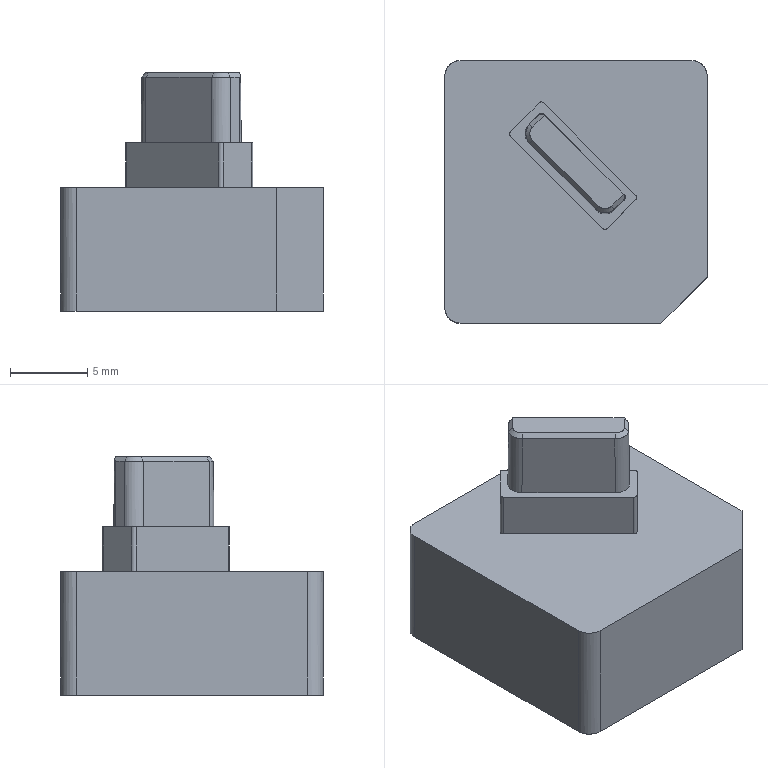NC program | PowerMill | posted with a generic post | part box 17 x 17 x 15.424 mm
Lines 24578 to 24748 of 24748:
N24675 M6
N24676 S15000 M03
N24677 G00 G90 X0.0 Y0.0
N24678 G43 Z10.304 H13
N24679
N24680 G05 P10000 R8
N24681 X-7.0637 Y-6.5861
N24682 Z-7.57
N24683 G01 Z-7.67
N24684 X-7.2667 Y-6.5717 F1000.0
N24685 X-7.4246 Y-6.5286
N24686 X-7.5373 Y-6.4567
N24687 X-7.605 Y-6.3559
N24688 X-7.6276 Y-6.2265
N24689 X-7.605 Y-6.097
N24690 X-7.5373 Y-5.9963
N24691 X-7.4246 Y-5.9244
N24692 X-7.2667 Y-5.8812
N24693 X-7.0637 Y-5.8668
N24694 X-6.8452 Y-5.8845
N24695 X-6.6794 Y-5.9378
N24696 X-6.5662 Y-6.0265
N24697 X-6.5177 Y-6.116
N24698 X-6.5015 Y-6.2265
N24699 X-6.524 Y-6.3559
N24700 X-6.5915 Y-6.4567
N24701 X-6.7039 Y-6.5286
N24702 X-6.8613 Y-6.5717
N24703 X-7.0637 Y-6.5861
N24704 G00 Z-4.4979
N24705 G01 X-6.5133 Y-4.8376 F10000.0
N24706 G00 Z-7.57
N24707 G01 Z-7.67 F600.0
N24708 X-7.6276 Y-4.8384 F1000.0
N24709 X-6.7889 Y-5.4519
N24710 Y-4.7224
N24711 G00 Z-4.4979
N24712 G01 X-6.9091 Y-3.805 F10000.0
N24713 G00 Z-7.57
N24714 G01 Z-7.67 F600.0
N24715 Y-4.2277 F1000.0
N24716 G00 Z-4.4979
N24717 G01 X-6.8696 Y-2.3732 F10000.0
N24718 G00 Z-7.57
N24719 G01 Z-7.67 F600.0
N24720 X-6.7152 Y-2.4356 F1000.0
N24721 X-6.5998 Y-2.5337
N24722 X-6.5261 Y-2.6669
N24723 X-6.5015 Y-2.8295
N24724 X-6.5329 Y-3.0323
N24725 X-6.627 Y-3.1858
N24726 X-6.7839 Y-3.29
N24727 X-6.9263 Y-3.3335
N24728 X-7.0797 Y-3.348
N24729 X-7.293 Y-3.3199
N24730 X-7.458 Y-3.2356
N24731 X-7.5746 Y-3.0951
N24732 X-7.625 Y-2.9673
N24733 X-7.6419 Y-2.8278
N24734 X-7.6212 Y-2.6766
N24735 X-7.5591 Y-2.5505
N24736 X-7.4579 Y-2.4541
N24737 X-7.32 Y-2.3917
N24738 G00 Z-4.4979
N24739 G01 X-7.2667 Y-1.901 F10000.0
N24740 G00 Z-7.57
N24741 G01 Z-7.67 F600.0
N24742 X-7.4246 Y-1.8578 F1000.0
N24743 X-7.5373 Y-1.7859
N24744 X-7.605 Y-1.6852
N24745 X-7.6276 Y-1.5557
N24746 X-7.605 Y-1.4262
N24747 X-7.5373 Y-1.3255
N24748 X-7.4246 Y-1.2536
N24749 X-7.2667 Y-1.2104
N24750 X-7.0637 Y-1.1961
N24751 X-6.8452 Y-1.2138
N24752 X-6.6794 Y-1.267
N24753 X-6.5662 Y-1.3557
N24754 X-6.5177 Y-1.4452
N24755 X-6.5015 Y-1.5557
N24756 X-6.524 Y-1.6852
N24757 X-6.5915 Y-1.7859
N24758 X-6.7039 Y-1.8578
N24759 X-6.8613 Y-1.901
N24760 X-7.0637 Y-1.9154
N24761 X-7.2667 Y-1.901
N24762 G00 Z-4.4979
N24763 G01 X-7.4797 Y-0.424 F10000.0
N24764 G00 Z-7.57
N24765 G01 Z-7.67 F600.0
N24766 X-7.6225 Y-0.2164 F1000.0
N24767 X-6.52
N24768 G00 Z-4.4979
N24769 G01 X-6.9091 Y0.8658 F10000.0
N24770 G00 Z-7.57
N24771 G01 Z-7.67 F600.0
N24772 Y0.4431 F1000.0
N24773 G00 Z-4.4979
N24774 G01 X-6.5133 Y1.869 F10000.0
N24775 G00 Z-7.57
N24776 G01 Z-7.67 F600.0
N24777 X-7.6276 Y1.8681 F1000.0
N24778 X-6.7889 Y1.2547
N24779 Y1.9841
N24780 G00 Z-4.4979
N24781 G01 X-6.9091 Y2.9016 F10000.0
N24782 G00 Z-7.57
N24783 G01 Z-7.67 F600.0
N24784 Y2.4789 F1000.0
N24785 G00 Z-4.4979
N24786 G01 X-6.9712 Y3.3525 F10000.0
N24787 G00 Z-7.57
N24788 G01 Z-7.67 F600.0
N24789 X-7.0637 Y3.3459 F1000.0
N24790 X-7.2667 Y3.3603
N24791 X-7.4246 Y3.4035
N24792 X-7.5373 Y3.4754
N24793 X-7.605 Y3.5761
N24794 X-7.6276 Y3.7056
N24795 X-7.605 Y3.8351
N24796 X-7.5373 Y3.9358
N24797 X-7.4246 Y4.0077
N24798 X-7.2667 Y4.0509
N24799 X-7.0637 Y4.0653
N24800 X-6.8452 Y4.0475
N24801 X-6.6794 Y3.9943
N24802 X-6.5662 Y3.9056
N24803 X-6.5177 Y3.8161
N24804 X-6.5015 Y3.7056
N24805 X-6.524 Y3.5761
N24806 X-6.5915 Y3.4754
N24807 X-6.7039 Y3.4035
N24808 X-6.8613 Y3.3603
N24809 X-6.9712 Y3.3525
N24810 G00 Z-4.4979
N24811 G01 X-6.5755 Y4.6794 F10000.0
N24812 G00 Z-7.57
N24813 G01 Z-7.67 F600.0
N24814 X-6.7281 F1000.0
N24815 G00 Z-4.4979
N24816 G01 X-7.3082 Y5.3044 F10000.0
N24817 G00 Z-7.57
N24818 G01 Z-7.67 F600.0
N24819 X-7.4448 Y5.3386 F1000.0
N24820 X-7.5452 Y5.4124
N24821 X-7.607 Y5.522
N24822 X-7.6276 Y5.6632
N24823 X-7.6078 Y5.7962
N24824 X-7.5486 Y5.9044
N24825 X-7.4492 Y5.9813
N24826 X-7.3208 Y6.0069
N24827 X-7.2469 Y5.9956
N24828 X-7.1713 Y5.9616
N24829 X-7.0704 Y5.8658
N24830 X-7.0412 Y5.817
N24831 X-6.9322 Y5.5674
N24832 X-6.8259 Y5.4321
N24833 X-6.6813 Y5.3254
N24834 X-6.52 Y5.2792
N24835 Y6.0078
N24836 G00 Z10.304
N24837 G05 P0
N24838 (---------------)
N24839 ( END TOOLPATH : 粗公刻字01-刻字-TEXT_D4 )
N24840 (---------------)
N24841
N24842 M05
N24843 G53 Z0.0
N24844 M30
%